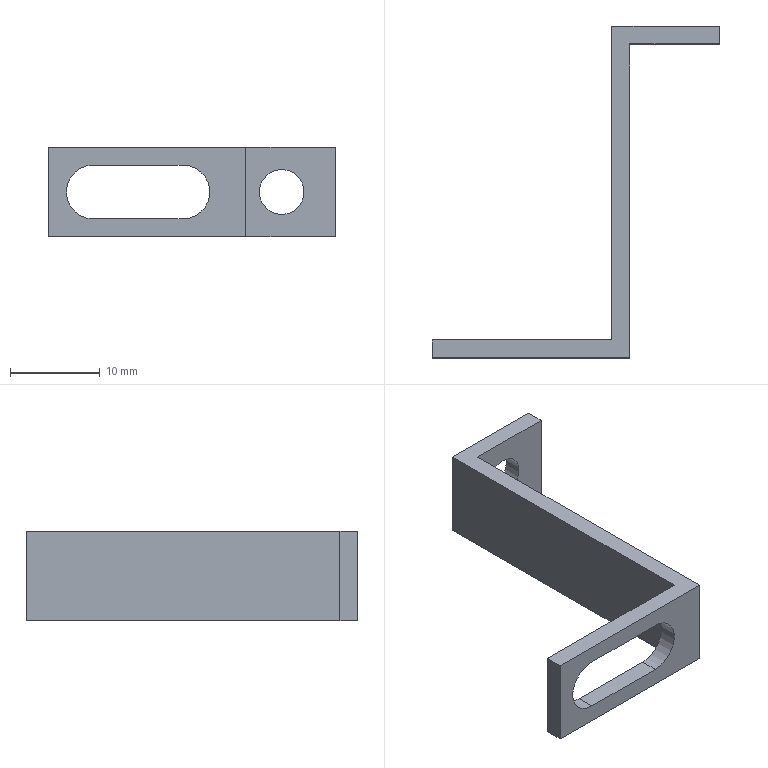Part | STEP file | Guide wheel mechanism revised.sldasm-Part-404 | 1 solid | 16 faces | box 32 x 37 x 10 mm | volume 1124 mm3 | plane 12 | cylinder 4 | commonest cylinder face diameters 5 x2 6 x2
STEP:
#1=CARTESIAN_POINT('',(6.,33.,-2.5));
#2=VERTEX_POINT('',#1);
#3=CARTESIAN_POINT('',(6.,33.,2.5));
#4=VERTEX_POINT('',#3);
#5=CARTESIAN_POINT('',(6.,33.,0.));
#6=DIRECTION('',(0.,1.,0.));
#7=DIRECTION('',(0.,0.,1.));
#8=AXIS2_PLACEMENT_3D('',#5,#6,#7);
#9=CIRCLE('',#8,2.5);
#10=EDGE_CURVE('',#2,#4,#9,.T.);
#11=ORIENTED_EDGE('',*,*,#10,.F.);
#12=CARTESIAN_POINT('',(6.,35.,-2.5));
#13=VERTEX_POINT('',#12);
#14=CARTESIAN_POINT('',(6.,-19.088,-2.5));
#15=DIRECTION('',(0.,1.,0.));
#16=VECTOR('',#15,1000.);
#17=LINE('',#14,#16);
#18=EDGE_CURVE('',#2,#13,#17,.T.);
#19=ORIENTED_EDGE('',*,*,#18,.T.);
#20=CARTESIAN_POINT('',(6.,35.,2.5));
#21=VERTEX_POINT('',#20);
#22=CARTESIAN_POINT('',(6.,35.,0.));
#23=DIRECTION('',(0.,1.,0.));
#24=DIRECTION('',(0.,0.,1.));
#25=AXIS2_PLACEMENT_3D('',#22,#23,#24);
#26=CIRCLE('',#25,2.5);
#27=EDGE_CURVE('',#13,#21,#26,.T.);
#28=ORIENTED_EDGE('',*,*,#27,.T.);
#29=CARTESIAN_POINT('',(6.,-19.088,2.5));
#30=DIRECTION('',(0.,1.,0.));
#31=VECTOR('',#30,1000.);
#32=LINE('',#29,#31);
#33=EDGE_CURVE('',#4,#21,#32,.T.);
#34=ORIENTED_EDGE('',*,*,#33,.F.);
#35=EDGE_LOOP('',(#11,#19,#28,#34));
#36=FACE_OUTER_BOUND('',#35,.T.);
#37=CARTESIAN_POINT('',(6.,-19.088,0.));
#38=DIRECTION('',(0.,1.,0.));
#39=DIRECTION('',(0.,0.,1.));
#40=AXIS2_PLACEMENT_3D('',#37,#38,#39);
#41=CYLINDRICAL_SURFACE('',#40,2.5);
#42=ADVANCED_FACE('',(#36),#41,.F.);
#43=CARTESIAN_POINT('',(6.,33.,0.));
#44=DIRECTION('',(0.,1.,0.));
#45=DIRECTION('',(0.,0.,1.));
#46=AXIS2_PLACEMENT_3D('',#43,#44,#45);
#47=CIRCLE('',#46,2.5);
#48=EDGE_CURVE('',#4,#2,#47,.T.);
#49=ORIENTED_EDGE('',*,*,#48,.T.);
#50=ORIENTED_EDGE('',*,*,#10,.T.);
#51=EDGE_LOOP('',(#49,#50));
#52=FACE_BOUND('',#51,.T.);
#53=CARTESIAN_POINT('',(2.,33.,-5.));
#54=VERTEX_POINT('',#53);
#55=CARTESIAN_POINT('',(12.,33.,-5.));
#56=VERTEX_POINT('',#55);
#57=CARTESIAN_POINT('',(0.,33.,-5.));
#58=DIRECTION('',(1.,0.,0.));
#59=VECTOR('',#58,1000.);
#60=LINE('',#57,#59);
#61=EDGE_CURVE('',#54,#56,#60,.T.);
#62=ORIENTED_EDGE('',*,*,#61,.T.);
#63=CARTESIAN_POINT('',(12.,33.,5.));
#64=VERTEX_POINT('',#63);
#65=CARTESIAN_POINT('',(12.,33.,5.));
#66=DIRECTION('',(0.,0.,-1.));
#67=VECTOR('',#66,1000.);
#68=LINE('',#65,#67);
#69=EDGE_CURVE('',#64,#56,#68,.T.);
#70=ORIENTED_EDGE('',*,*,#69,.F.);
#71=CARTESIAN_POINT('',(2.,33.,5.));
#72=VERTEX_POINT('',#71);
#73=CARTESIAN_POINT('',(0.,33.,5.));
#74=DIRECTION('',(1.,0.,0.));
#75=VECTOR('',#74,1000.);
#76=LINE('',#73,#75);
#77=EDGE_CURVE('',#72,#64,#76,.T.);
#78=ORIENTED_EDGE('',*,*,#77,.F.);
#79=CARTESIAN_POINT('',(2.,33.,5.));
#80=DIRECTION('',(0.,0.,-1.));
#81=VECTOR('',#80,1000.);
#82=LINE('',#79,#81);
#83=EDGE_CURVE('',#72,#54,#82,.T.);
#84=ORIENTED_EDGE('',*,*,#83,.T.);
#85=EDGE_LOOP('',(#62,#70,#78,#84));
#86=FACE_OUTER_BOUND('',#85,.T.);
#87=CARTESIAN_POINT('',(0.,33.,5.));
#88=DIRECTION('',(0.,1.,0.));
#89=DIRECTION('',(0.,0.,1.));
#90=AXIS2_PLACEMENT_3D('',#87,#88,#89);
#91=PLANE('',#90);
#92=ADVANCED_FACE('',(#52,#86),#91,.F.);
#93=CARTESIAN_POINT('',(12.,35.,-5.));
#94=VERTEX_POINT('',#93);
#95=CARTESIAN_POINT('',(12.,35.,-5.));
#96=DIRECTION('',(0.,-1.,0.));
#97=VECTOR('',#96,1000.);
#98=LINE('',#95,#97);
#99=EDGE_CURVE('',#94,#56,#98,.T.);
#100=ORIENTED_EDGE('',*,*,#99,.F.);
#101=CARTESIAN_POINT('',(12.,35.,5.));
#102=VERTEX_POINT('',#101);
#103=CARTESIAN_POINT('',(12.,35.,5.));
#104=DIRECTION('',(0.,0.,-1.));
#105=VECTOR('',#104,1000.);
#106=LINE('',#103,#105);
#107=EDGE_CURVE('',#102,#94,#106,.T.);
#108=ORIENTED_EDGE('',*,*,#107,.F.);
#109=CARTESIAN_POINT('',(12.,35.,5.));
#110=DIRECTION('',(0.,-1.,0.));
#111=VECTOR('',#110,1000.);
#112=LINE('',#109,#111);
#113=EDGE_CURVE('',#102,#64,#112,.T.);
#114=ORIENTED_EDGE('',*,*,#113,.T.);
#115=ORIENTED_EDGE('',*,*,#69,.T.);
#116=EDGE_LOOP('',(#100,#108,#114,#115));
#117=FACE_OUTER_BOUND('',#116,.T.);
#118=CARTESIAN_POINT('',(12.,35.,5.));
#119=DIRECTION('',(1.,0.,0.));
#120=DIRECTION('',(0.,0.,-1.));
#121=AXIS2_PLACEMENT_3D('',#118,#119,#120);
#122=PLANE('',#121);
#123=ADVANCED_FACE('',(#117),#122,.T.);
#124=CARTESIAN_POINT('',(6.,35.,0.));
#125=DIRECTION('',(0.,1.,0.));
#126=DIRECTION('',(0.,0.,1.));
#127=AXIS2_PLACEMENT_3D('',#124,#125,#126);
#128=CIRCLE('',#127,2.5);
#129=EDGE_CURVE('',#21,#13,#128,.T.);
#130=ORIENTED_EDGE('',*,*,#129,.F.);
#131=ORIENTED_EDGE('',*,*,#27,.F.);
#132=EDGE_LOOP('',(#130,#131));
#133=FACE_BOUND('',#132,.T.);
#134=CARTESIAN_POINT('',(0.,35.,-5.));
#135=VERTEX_POINT('',#134);
#136=CARTESIAN_POINT('',(0.,35.,-5.));
#137=DIRECTION('',(1.,0.,0.));
#138=VECTOR('',#137,1000.);
#139=LINE('',#136,#138);
#140=EDGE_CURVE('',#135,#94,#139,.T.);
#141=ORIENTED_EDGE('',*,*,#140,.F.);
#142=CARTESIAN_POINT('',(0.,35.,5.));
#143=VERTEX_POINT('',#142);
#144=CARTESIAN_POINT('',(0.,35.,5.));
#145=DIRECTION('',(0.,0.,-1.));
#146=VECTOR('',#145,1000.);
#147=LINE('',#144,#146);
#148=EDGE_CURVE('',#143,#135,#147,.T.);
#149=ORIENTED_EDGE('',*,*,#148,.F.);
#150=CARTESIAN_POINT('',(0.,35.,5.));
#151=DIRECTION('',(1.,0.,0.));
#152=VECTOR('',#151,1000.);
#153=LINE('',#150,#152);
#154=EDGE_CURVE('',#143,#102,#153,.T.);
#155=ORIENTED_EDGE('',*,*,#154,.T.);
#156=ORIENTED_EDGE('',*,*,#107,.T.);
#157=EDGE_LOOP('',(#141,#149,#155,#156));
#158=FACE_OUTER_BOUND('',#157,.T.);
#159=CARTESIAN_POINT('',(0.,35.,5.));
#160=DIRECTION('',(0.,1.,0.));
#161=DIRECTION('',(0.,0.,1.));
#162=AXIS2_PLACEMENT_3D('',#159,#160,#161);
#163=PLANE('',#162);
#164=ADVANCED_FACE('',(#133,#158),#163,.T.);
#165=CARTESIAN_POINT('',(0.,0.,-5.));
#166=VERTEX_POINT('',#165);
#167=CARTESIAN_POINT('',(0.,0.,-5.));
#168=DIRECTION('',(0.,1.,0.));
#169=VECTOR('',#168,1000.);
#170=LINE('',#167,#169);
#171=EDGE_CURVE('',#166,#135,#170,.T.);
#172=ORIENTED_EDGE('',*,*,#171,.F.);
#173=CARTESIAN_POINT('',(0.,0.,5.));
#174=VERTEX_POINT('',#173);
#175=CARTESIAN_POINT('',(0.,0.,5.));
#176=DIRECTION('',(0.,0.,-1.));
#177=VECTOR('',#176,1000.);
#178=LINE('',#175,#177);
#179=EDGE_CURVE('',#174,#166,#178,.T.);
#180=ORIENTED_EDGE('',*,*,#179,.F.);
#181=CARTESIAN_POINT('',(0.,0.,5.));
#182=DIRECTION('',(0.,1.,0.));
#183=VECTOR('',#182,1000.);
#184=LINE('',#181,#183);
#185=EDGE_CURVE('',#174,#143,#184,.T.);
#186=ORIENTED_EDGE('',*,*,#185,.T.);
#187=ORIENTED_EDGE('',*,*,#148,.T.);
#188=EDGE_LOOP('',(#172,#180,#186,#187));
#189=FACE_OUTER_BOUND('',#188,.T.);
#190=CARTESIAN_POINT('',(0.,0.,5.));
#191=DIRECTION('',(-1.,0.,0.));
#192=DIRECTION('',(0.,0.,1.));
#193=AXIS2_PLACEMENT_3D('',#190,#191,#192);
#194=PLANE('',#193);
#195=ADVANCED_FACE('',(#189),#194,.T.);
#196=CARTESIAN_POINT('',(-5.,0.,3.));
#197=VERTEX_POINT('',#196);
#198=CARTESIAN_POINT('',(-5.,0.,-3.));
#199=VERTEX_POINT('',#198);
#200=CARTESIAN_POINT('',(-5.,0.,0.));
#201=DIRECTION('',(0.,1.,0.));
#202=DIRECTION('',(-1.,0.,0.));
#203=AXIS2_PLACEMENT_3D('',#200,#201,#202);
#204=CIRCLE('',#203,3.);
#205=EDGE_CURVE('',#197,#199,#204,.T.);
#206=ORIENTED_EDGE('',*,*,#205,.F.);
#207=CARTESIAN_POINT('',(-15.,0.,3.));
#208=VERTEX_POINT('',#207);
#209=CARTESIAN_POINT('',(0.,0.,3.));
#210=DIRECTION('',(1.,0.,0.));
#211=VECTOR('',#210,1000.);
#212=LINE('',#209,#211);
#213=EDGE_CURVE('',#208,#197,#212,.T.);
#214=ORIENTED_EDGE('',*,*,#213,.F.);
#215=CARTESIAN_POINT('',(-15.,0.,-3.));
#216=VERTEX_POINT('',#215);
#217=CARTESIAN_POINT('',(-15.,0.,0.));
#218=DIRECTION('',(0.,1.,0.));
#219=DIRECTION('',(-1.,0.,0.));
#220=AXIS2_PLACEMENT_3D('',#217,#218,#219);
#221=CIRCLE('',#220,3.);
#222=EDGE_CURVE('',#216,#208,#221,.T.);
#223=ORIENTED_EDGE('',*,*,#222,.F.);
#224=CARTESIAN_POINT('',(0.,0.,-3.));
#225=DIRECTION('',(-1.,0.,0.));
#226=VECTOR('',#225,1000.);
#227=LINE('',#224,#226);
#228=EDGE_CURVE('',#199,#216,#227,.T.);
#229=ORIENTED_EDGE('',*,*,#228,.F.);
#230=EDGE_LOOP('',(#206,#214,#223,#229));
#231=FACE_BOUND('',#230,.T.);
#232=CARTESIAN_POINT('',(-20.,0.,-5.));
#233=VERTEX_POINT('',#232);
#234=CARTESIAN_POINT('',(0.,0.,-5.));
#235=DIRECTION('',(1.,0.,0.));
#236=VECTOR('',#235,1000.);
#237=LINE('',#234,#236);
#238=EDGE_CURVE('',#233,#166,#237,.T.);
#239=ORIENTED_EDGE('',*,*,#238,.F.);
#240=CARTESIAN_POINT('',(-20.,0.,5.));
#241=VERTEX_POINT('',#240);
#242=CARTESIAN_POINT('',(-20.,0.,5.));
#243=DIRECTION('',(0.,0.,-1.));
#244=VECTOR('',#243,1000.);
#245=LINE('',#242,#244);
#246=EDGE_CURVE('',#241,#233,#245,.T.);
#247=ORIENTED_EDGE('',*,*,#246,.F.);
#248=CARTESIAN_POINT('',(0.,0.,5.));
#249=DIRECTION('',(1.,0.,0.));
#250=VECTOR('',#249,1000.);
#251=LINE('',#248,#250);
#252=EDGE_CURVE('',#241,#174,#251,.T.);
#253=ORIENTED_EDGE('',*,*,#252,.T.);
#254=ORIENTED_EDGE('',*,*,#179,.T.);
#255=EDGE_LOOP('',(#239,#247,#253,#254));
#256=FACE_OUTER_BOUND('',#255,.T.);
#257=CARTESIAN_POINT('',(0.,0.,5.));
#258=DIRECTION('',(0.,1.,0.));
#259=DIRECTION('',(-1.,0.,0.));
#260=AXIS2_PLACEMENT_3D('',#257,#258,#259);
#261=PLANE('',#260);
#262=ADVANCED_FACE('',(#231,#256),#261,.T.);
#263=CARTESIAN_POINT('',(-20.,-2.,-5.));
#264=VERTEX_POINT('',#263);
#265=CARTESIAN_POINT('',(-20.,-2.,-5.));
#266=DIRECTION('',(0.,1.,0.));
#267=VECTOR('',#266,1000.);
#268=LINE('',#265,#267);
#269=EDGE_CURVE('',#264,#233,#268,.T.);
#270=ORIENTED_EDGE('',*,*,#269,.F.);
#271=CARTESIAN_POINT('',(-20.,-2.,5.));
#272=VERTEX_POINT('',#271);
#273=CARTESIAN_POINT('',(-20.,-2.,5.));
#274=DIRECTION('',(0.,0.,-1.));
#275=VECTOR('',#274,1000.);
#276=LINE('',#273,#275);
#277=EDGE_CURVE('',#272,#264,#276,.T.);
#278=ORIENTED_EDGE('',*,*,#277,.F.);
#279=CARTESIAN_POINT('',(-20.,-2.,5.));
#280=DIRECTION('',(0.,1.,0.));
#281=VECTOR('',#280,1000.);
#282=LINE('',#279,#281);
#283=EDGE_CURVE('',#272,#241,#282,.T.);
#284=ORIENTED_EDGE('',*,*,#283,.T.);
#285=ORIENTED_EDGE('',*,*,#246,.T.);
#286=EDGE_LOOP('',(#270,#278,#284,#285));
#287=FACE_OUTER_BOUND('',#286,.T.);
#288=CARTESIAN_POINT('',(-20.,-2.,5.));
#289=DIRECTION('',(-1.,0.,0.));
#290=DIRECTION('',(0.,0.,1.));
#291=AXIS2_PLACEMENT_3D('',#288,#289,#290);
#292=PLANE('',#291);
#293=ADVANCED_FACE('',(#287),#292,.T.);
#294=CARTESIAN_POINT('',(-5.,-2.,3.));
#295=VERTEX_POINT('',#294);
#296=CARTESIAN_POINT('',(-15.,-2.,3.));
#297=VERTEX_POINT('',#296);
#298=CARTESIAN_POINT('',(-5.,-2.,3.));
#299=DIRECTION('',(-1.,0.,0.));
#300=VECTOR('',#299,1000.);
#301=LINE('',#298,#300);
#302=EDGE_CURVE('',#295,#297,#301,.T.);
#303=ORIENTED_EDGE('',*,*,#302,.F.);
#304=CARTESIAN_POINT('',(-5.,-2.,-3.));
#305=VERTEX_POINT('',#304);
#306=CARTESIAN_POINT('',(-5.,-2.,0.));
#307=DIRECTION('',(0.,-1.,0.));
#308=DIRECTION('',(-1.,0.,0.));
#309=AXIS2_PLACEMENT_3D('',#306,#307,#308);
#310=CIRCLE('',#309,3.);
#311=EDGE_CURVE('',#305,#295,#310,.T.);
#312=ORIENTED_EDGE('',*,*,#311,.F.);
#313=CARTESIAN_POINT('',(-15.,-2.,-3.));
#314=VERTEX_POINT('',#313);
#315=CARTESIAN_POINT('',(-5.,-2.,-3.));
#316=DIRECTION('',(1.,0.,0.));
#317=VECTOR('',#316,1000.);
#318=LINE('',#315,#317);
#319=EDGE_CURVE('',#314,#305,#318,.T.);
#320=ORIENTED_EDGE('',*,*,#319,.F.);
#321=CARTESIAN_POINT('',(-15.,-2.,0.));
#322=DIRECTION('',(0.,-1.,0.));
#323=DIRECTION('',(-1.,0.,0.));
#324=AXIS2_PLACEMENT_3D('',#321,#322,#323);
#325=CIRCLE('',#324,3.);
#326=EDGE_CURVE('',#297,#314,#325,.T.);
#327=ORIENTED_EDGE('',*,*,#326,.F.);
#328=EDGE_LOOP('',(#303,#312,#320,#327));
#329=FACE_BOUND('',#328,.T.);
#330=CARTESIAN_POINT('',(2.,-2.,-5.));
#331=VERTEX_POINT('',#330);
#332=CARTESIAN_POINT('',(0.,-2.,-5.));
#333=DIRECTION('',(1.,0.,0.));
#334=VECTOR('',#333,1000.);
#335=LINE('',#332,#334);
#336=EDGE_CURVE('',#264,#331,#335,.T.);
#337=ORIENTED_EDGE('',*,*,#336,.T.);
#338=CARTESIAN_POINT('',(2.,-2.,5.));
#339=VERTEX_POINT('',#338);
#340=CARTESIAN_POINT('',(2.,-2.,5.));
#341=DIRECTION('',(0.,0.,-1.));
#342=VECTOR('',#341,1000.);
#343=LINE('',#340,#342);
#344=EDGE_CURVE('',#339,#331,#343,.T.);
#345=ORIENTED_EDGE('',*,*,#344,.F.);
#346=CARTESIAN_POINT('',(0.,-2.,5.));
#347=DIRECTION('',(1.,0.,0.));
#348=VECTOR('',#347,1000.);
#349=LINE('',#346,#348);
#350=EDGE_CURVE('',#272,#339,#349,.T.);
#351=ORIENTED_EDGE('',*,*,#350,.F.);
#352=ORIENTED_EDGE('',*,*,#277,.T.);
#353=EDGE_LOOP('',(#337,#345,#351,#352));
#354=FACE_OUTER_BOUND('',#353,.T.);
#355=CARTESIAN_POINT('',(0.,-2.,5.));
#356=DIRECTION('',(0.,1.,0.));
#357=DIRECTION('',(-1.,0.,0.));
#358=AXIS2_PLACEMENT_3D('',#355,#356,#357);
#359=PLANE('',#358);
#360=ADVANCED_FACE('',(#329,#354),#359,.F.);
#361=CARTESIAN_POINT('',(2.,0.,-5.));
#362=DIRECTION('',(0.,1.,0.));
#363=VECTOR('',#362,1000.);
#364=LINE('',#361,#363);
#365=EDGE_CURVE('',#331,#54,#364,.T.);
#366=ORIENTED_EDGE('',*,*,#365,.T.);
#367=ORIENTED_EDGE('',*,*,#83,.F.);
#368=CARTESIAN_POINT('',(2.,0.,5.));
#369=DIRECTION('',(0.,1.,0.));
#370=VECTOR('',#369,1000.);
#371=LINE('',#368,#370);
#372=EDGE_CURVE('',#339,#72,#371,.T.);
#373=ORIENTED_EDGE('',*,*,#372,.F.);
#374=ORIENTED_EDGE('',*,*,#344,.T.);
#375=EDGE_LOOP('',(#366,#367,#373,#374));
#376=FACE_OUTER_BOUND('',#375,.T.);
#377=CARTESIAN_POINT('',(2.,0.,5.));
#378=DIRECTION('',(-1.,0.,0.));
#379=DIRECTION('',(0.,0.,1.));
#380=AXIS2_PLACEMENT_3D('',#377,#378,#379);
#381=PLANE('',#380);
#382=ADVANCED_FACE('',(#376),#381,.F.);
#383=ORIENTED_EDGE('',*,*,#77,.T.);
#384=ORIENTED_EDGE('',*,*,#113,.F.);
#385=ORIENTED_EDGE('',*,*,#154,.F.);
#386=ORIENTED_EDGE('',*,*,#185,.F.);
#387=ORIENTED_EDGE('',*,*,#252,.F.);
#388=ORIENTED_EDGE('',*,*,#283,.F.);
#389=ORIENTED_EDGE('',*,*,#350,.T.);
#390=ORIENTED_EDGE('',*,*,#372,.T.);
#391=EDGE_LOOP('',(#383,#384,#385,#386,#387,#388,#389,#390));
#392=FACE_OUTER_BOUND('',#391,.T.);
#393=CARTESIAN_POINT('',(0.,0.,5.));
#394=DIRECTION('',(0.,0.,-1.));
#395=DIRECTION('',(-1.,0.,0.));
#396=AXIS2_PLACEMENT_3D('',#393,#394,#395);
#397=PLANE('',#396);
#398=ADVANCED_FACE('',(#392),#397,.F.);
#399=ORIENTED_EDGE('',*,*,#61,.F.);
#400=ORIENTED_EDGE('',*,*,#365,.F.);
#401=ORIENTED_EDGE('',*,*,#336,.F.);
#402=ORIENTED_EDGE('',*,*,#269,.T.);
#403=ORIENTED_EDGE('',*,*,#238,.T.);
#404=ORIENTED_EDGE('',*,*,#171,.T.);
#405=ORIENTED_EDGE('',*,*,#140,.T.);
#406=ORIENTED_EDGE('',*,*,#99,.T.);
#407=EDGE_LOOP('',(#399,#400,#401,#402,#403,#404,#405,#406));
#408=FACE_OUTER_BOUND('',#407,.T.);
#409=CARTESIAN_POINT('',(0.,0.,-5.));
#410=DIRECTION('',(0.,0.,-1.));
#411=DIRECTION('',(-1.,0.,0.));
#412=AXIS2_PLACEMENT_3D('',#409,#410,#411);
#413=PLANE('',#412);
#414=ADVANCED_FACE('',(#408),#413,.T.);
#415=ORIENTED_EDGE('',*,*,#18,.F.);
#416=ORIENTED_EDGE('',*,*,#48,.F.);
#417=ORIENTED_EDGE('',*,*,#33,.T.);
#418=ORIENTED_EDGE('',*,*,#129,.T.);
#419=EDGE_LOOP('',(#415,#416,#417,#418));
#420=FACE_OUTER_BOUND('',#419,.T.);
#421=CARTESIAN_POINT('',(6.,-19.088,0.));
#422=DIRECTION('',(0.,1.,0.));
#423=DIRECTION('',(0.,0.,1.));
#424=AXIS2_PLACEMENT_3D('',#421,#422,#423);
#425=CYLINDRICAL_SURFACE('',#424,2.5);
#426=ADVANCED_FACE('',(#420),#425,.F.);
#427=ORIENTED_EDGE('',*,*,#205,.T.);
#428=CARTESIAN_POINT('',(-5.,-19.088,-3.));
#429=DIRECTION('',(0.,1.,0.));
#430=VECTOR('',#429,1000.);
#431=LINE('',#428,#430);
#432=EDGE_CURVE('',#305,#199,#431,.T.);
#433=ORIENTED_EDGE('',*,*,#432,.F.);
#434=ORIENTED_EDGE('',*,*,#311,.T.);
#435=CARTESIAN_POINT('',(-5.,-19.088,3.));
#436=DIRECTION('',(0.,1.,0.));
#437=VECTOR('',#436,1000.);
#438=LINE('',#435,#437);
#439=EDGE_CURVE('',#295,#197,#438,.T.);
#440=ORIENTED_EDGE('',*,*,#439,.T.);
#441=EDGE_LOOP('',(#427,#433,#434,#440));
#442=FACE_OUTER_BOUND('',#441,.T.);
#443=CARTESIAN_POINT('',(-5.,-19.088,0.));
#444=DIRECTION('',(0.,1.,0.));
#445=DIRECTION('',(0.,0.,1.));
#446=AXIS2_PLACEMENT_3D('',#443,#444,#445);
#447=CYLINDRICAL_SURFACE('',#446,3.);
#448=ADVANCED_FACE('',(#442),#447,.F.);
#449=ORIENTED_EDGE('',*,*,#213,.T.);
#450=ORIENTED_EDGE('',*,*,#439,.F.);
#451=ORIENTED_EDGE('',*,*,#302,.T.);
#452=CARTESIAN_POINT('',(-15.,-19.088,3.));
#453=DIRECTION('',(0.,1.,0.));
#454=VECTOR('',#453,1000.);
#455=LINE('',#452,#454);
#456=EDGE_CURVE('',#297,#208,#455,.T.);
#457=ORIENTED_EDGE('',*,*,#456,.T.);
#458=EDGE_LOOP('',(#449,#450,#451,#457));
#459=FACE_OUTER_BOUND('',#458,.T.);
#460=CARTESIAN_POINT('',(-5.,-19.088,3.));
#461=DIRECTION('',(0.,0.,1.));
#462=DIRECTION('',(1.,0.,0.));
#463=AXIS2_PLACEMENT_3D('',#460,#461,#462);
#464=PLANE('',#463);
#465=ADVANCED_FACE('',(#459),#464,.F.);
#466=ORIENTED_EDGE('',*,*,#222,.T.);
#467=ORIENTED_EDGE('',*,*,#456,.F.);
#468=ORIENTED_EDGE('',*,*,#326,.T.);
#469=CARTESIAN_POINT('',(-15.,-19.088,-3.));
#470=DIRECTION('',(0.,1.,0.));
#471=VECTOR('',#470,1000.);
#472=LINE('',#469,#471);
#473=EDGE_CURVE('',#314,#216,#472,.T.);
#474=ORIENTED_EDGE('',*,*,#473,.T.);
#475=EDGE_LOOP('',(#466,#467,#468,#474));
#476=FACE_OUTER_BOUND('',#475,.T.);
#477=CARTESIAN_POINT('',(-15.,-19.088,0.));
#478=DIRECTION('',(0.,1.,0.));
#479=DIRECTION('',(0.,0.,1.));
#480=AXIS2_PLACEMENT_3D('',#477,#478,#479);
#481=CYLINDRICAL_SURFACE('',#480,3.);
#482=ADVANCED_FACE('',(#476),#481,.F.);
#483=ORIENTED_EDGE('',*,*,#228,.T.);
#484=ORIENTED_EDGE('',*,*,#473,.F.);
#485=ORIENTED_EDGE('',*,*,#319,.T.);
#486=ORIENTED_EDGE('',*,*,#432,.T.);
#487=EDGE_LOOP('',(#483,#484,#485,#486));
#488=FACE_OUTER_BOUND('',#487,.T.);
#489=CARTESIAN_POINT('',(-5.,-19.088,-3.));
#490=DIRECTION('',(0.,0.,-1.));
#491=DIRECTION('',(-1.,0.,0.));
#492=AXIS2_PLACEMENT_3D('',#489,#490,#491);
#493=PLANE('',#492);
#494=ADVANCED_FACE('',(#488),#493,.F.);
#495=CLOSED_SHELL('',(#42,#92,#123,#164,#195,#262,#293,#360,#382,#398,#414,#426,#448,#465,#482,#494));
#496=MANIFOLD_SOLID_BREP('',#495);
#497=CARTESIAN_POINT('',(0.,0.,0.));
#498=DIRECTION('',(0.,0.,1.));
#499=DIRECTION('',(1.,0.,0.));
#500=AXIS2_PLACEMENT_3D('',#497,#498,#499);
#501=(LENGTH_UNIT()NAMED_UNIT(*)SI_UNIT(.MILLI.,.METRE.));
#502=UNCERTAINTY_MEASURE_WITH_UNIT(LENGTH_MEASURE(0.00001),#501,'','');
#503=(NAMED_UNIT(*)PLANE_ANGLE_UNIT()SI_UNIT($,.RADIAN.));
#504=(NAMED_UNIT(*)SI_UNIT($,.STERADIAN.)SOLID_ANGLE_UNIT());
#505=(GEOMETRIC_REPRESENTATION_CONTEXT(3)GLOBAL_UNCERTAINTY_ASSIGNED_CONTEXT((#502))GLOBAL_UNIT_ASSIGNED_CONTEXT((#501,#503,#504))REPRESENTATION_CONTEXT('',''));
#506=ADVANCED_BREP_SHAPE_REPRESENTATION('',(#496,#500),#505);